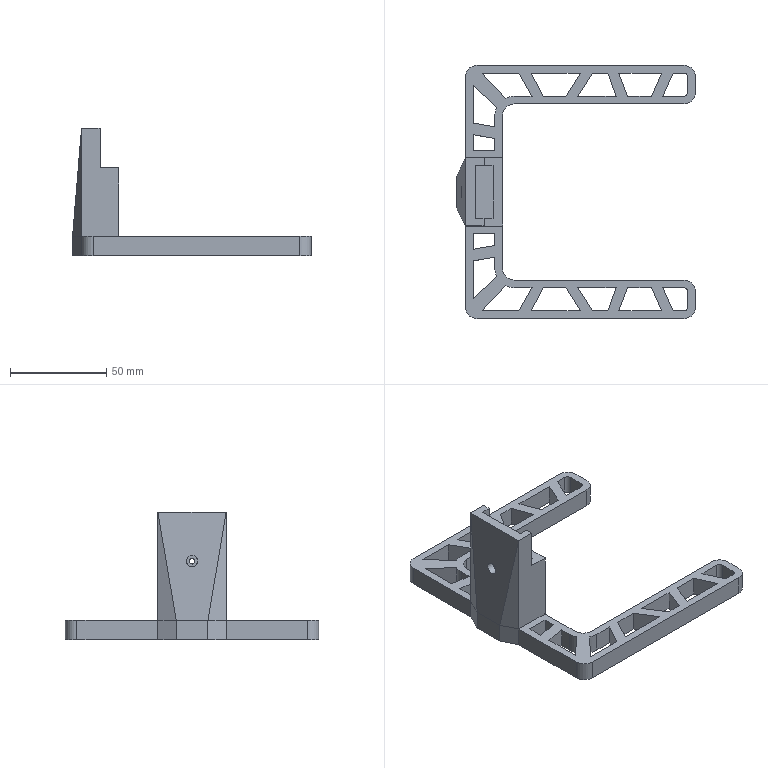Part | NX | features DATUM_CSYS 3, BREP 2, SKETCH 2 | 2 solids | 107 faces | box 123.846 x 131.35 x 66 mm | volume 70448 mm3 | plane 88 | cylinder 19 | commonest cylinder face diameters 12 x8 4 x4 20 x4 3 x2 5.85 x1